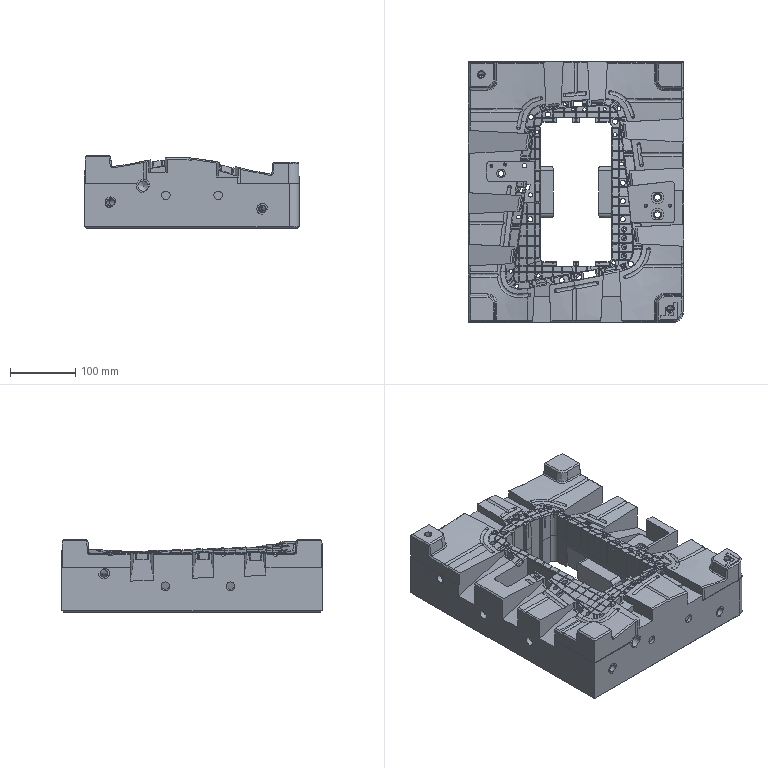Part | STEP file | P011002M001-000 | 1 solid | 3035 faces | volume 8732040 mm3 | spline 1131 | plane 1124 | other 313 | cone 282 | cylinder 185 | commonest cylinder face diameters 12 x37 6 x17 8 x14 9 x13 13 x11 5 x9